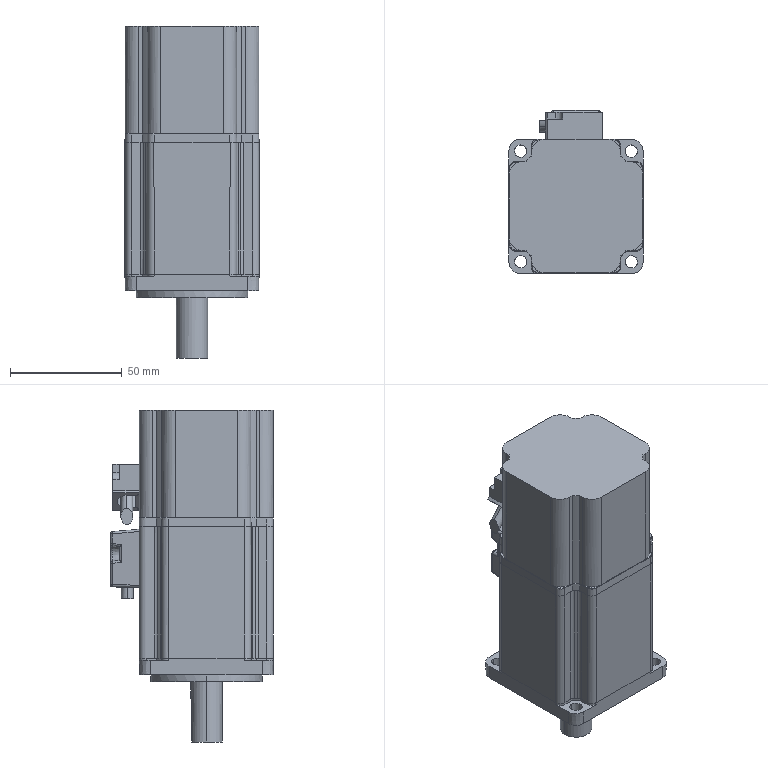Part | SolidWorks | features BaseBody 1 | 1 solid | 354 faces | box 60 x 72.85 x 148.5 mm | volume 399060 mm3 | plane 159 | cylinder 155 | spline 22 | cone 18 | commonest cylinder face diameters 6 x33 2 x20 0.6 x12 3 x8 3.3 x8 4 x8